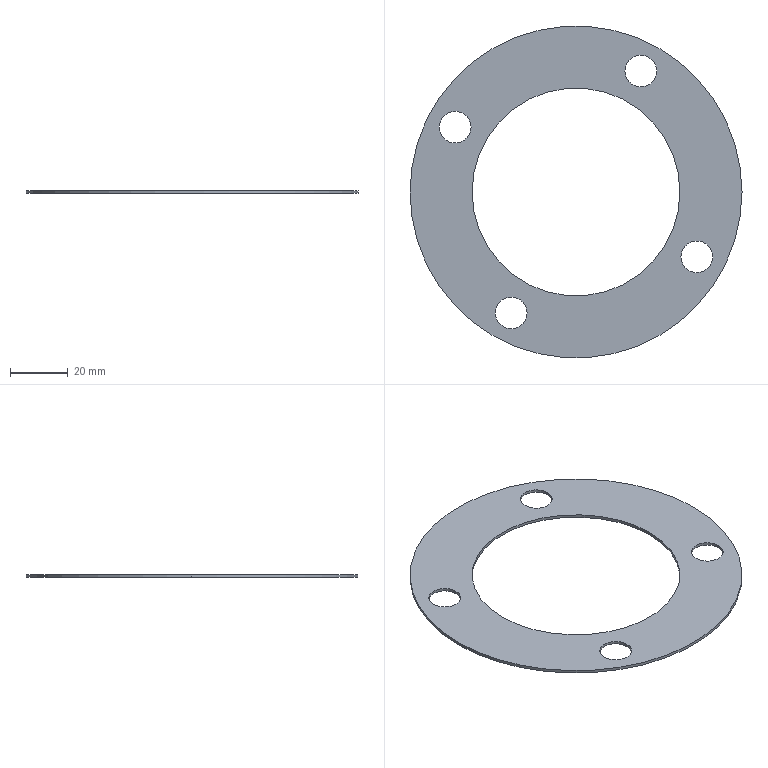Part | SolidWorks | features BaseBody 1 | 1 solid | 14 faces | box 115 x 115 x 1 mm | volume 5935 mm3 | cylinder 12 | plane 2 | commonest cylinder face diameters 11 x8 72 x2 115 x2
STEP:
#1=CARTESIAN_POINT('',(47.934,-43.434,0.));
#2=VERTEX_POINT('',#1);
#3=CARTESIAN_POINT('',(58.934,-43.434,0.));
#4=VERTEX_POINT('',#3);
#5=CARTESIAN_POINT('',(53.434,-43.434,0.));
#6=DIRECTION('',(0.,0.,1.));
#7=DIRECTION('',(1.,0.,0.));
#8=AXIS2_PLACEMENT_3D('',#5,#6,#7);
#9=CIRCLE('',#8,5.5);
#10=EDGE_CURVE('',#2,#4,#9,.T.);
#11=ORIENTED_EDGE('',*,*,#10,.F.);
#12=CARTESIAN_POINT('',(47.934,-43.434,1.));
#13=VERTEX_POINT('',#12);
#14=CARTESIAN_POINT('',(47.934,-43.434,0.));
#15=DIRECTION('',(0.,0.,1.));
#16=VECTOR('',#15,1000.);
#17=LINE('',#14,#16);
#18=EDGE_CURVE('',#2,#13,#17,.T.);
#19=ORIENTED_EDGE('',*,*,#18,.T.);
#20=CARTESIAN_POINT('',(58.934,-43.434,1.));
#21=VERTEX_POINT('',#20);
#22=CARTESIAN_POINT('',(53.434,-43.434,1.));
#23=DIRECTION('',(0.,0.,-1.));
#24=DIRECTION('',(1.,0.,0.));
#25=AXIS2_PLACEMENT_3D('',#22,#23,#24);
#26=CIRCLE('',#25,5.5);
#27=EDGE_CURVE('',#21,#13,#26,.T.);
#28=ORIENTED_EDGE('',*,*,#27,.F.);
#29=CARTESIAN_POINT('',(58.934,-43.434,0.));
#30=DIRECTION('',(0.,0.,1.));
#31=VECTOR('',#30,1000.);
#32=LINE('',#29,#31);
#33=EDGE_CURVE('',#4,#21,#32,.T.);
#34=ORIENTED_EDGE('',*,*,#33,.F.);
#35=EDGE_LOOP('',(#11,#19,#28,#34));
#36=FACE_OUTER_BOUND('',#35,.T.);
#37=CARTESIAN_POINT('',(53.434,-43.434,0.));
#38=DIRECTION('',(0.,0.,1.));
#39=DIRECTION('',(1.,0.,0.));
#40=AXIS2_PLACEMENT_3D('',#37,#38,#39);
#41=CYLINDRICAL_SURFACE('',#40,5.5);
#42=ADVANCED_FACE('',(#36),#41,.F.);
#43=CARTESIAN_POINT('',(112.242,-24.019,0.));
#44=VERTEX_POINT('',#43);
#45=CARTESIAN_POINT('',(123.242,-24.019,0.));
#46=VERTEX_POINT('',#45);
#47=CARTESIAN_POINT('',(117.742,-24.019,0.));
#48=DIRECTION('',(0.,0.,1.));
#49=DIRECTION('',(1.,0.,0.));
#50=AXIS2_PLACEMENT_3D('',#47,#48,#49);
#51=CIRCLE('',#50,5.5);
#52=EDGE_CURVE('',#44,#46,#51,.T.);
#53=ORIENTED_EDGE('',*,*,#52,.F.);
#54=CARTESIAN_POINT('',(112.242,-24.019,1.));
#55=VERTEX_POINT('',#54);
#56=CARTESIAN_POINT('',(112.242,-24.019,0.));
#57=DIRECTION('',(0.,0.,1.));
#58=VECTOR('',#57,1000.);
#59=LINE('',#56,#58);
#60=EDGE_CURVE('',#44,#55,#59,.T.);
#61=ORIENTED_EDGE('',*,*,#60,.T.);
#62=CARTESIAN_POINT('',(123.242,-24.019,1.));
#63=VERTEX_POINT('',#62);
#64=CARTESIAN_POINT('',(117.742,-24.019,1.));
#65=DIRECTION('',(0.,0.,-1.));
#66=DIRECTION('',(1.,0.,0.));
#67=AXIS2_PLACEMENT_3D('',#64,#65,#66);
#68=CIRCLE('',#67,5.5);
#69=EDGE_CURVE('',#63,#55,#68,.T.);
#70=ORIENTED_EDGE('',*,*,#69,.F.);
#71=CARTESIAN_POINT('',(123.242,-24.019,0.));
#72=DIRECTION('',(0.,0.,1.));
#73=VECTOR('',#72,1000.);
#74=LINE('',#71,#73);
#75=EDGE_CURVE('',#46,#63,#74,.T.);
#76=ORIENTED_EDGE('',*,*,#75,.F.);
#77=EDGE_LOOP('',(#53,#61,#70,#76));
#78=FACE_OUTER_BOUND('',#77,.T.);
#79=CARTESIAN_POINT('',(117.742,-24.019,0.));
#80=DIRECTION('',(0.,0.,1.));
#81=DIRECTION('',(1.,0.,0.));
#82=AXIS2_PLACEMENT_3D('',#79,#80,#81);
#83=CYLINDRICAL_SURFACE('',#82,5.5);
#84=ADVANCED_FACE('',(#78),#83,.F.);
#85=CARTESIAN_POINT('',(92.828,40.289,0.));
#86=VERTEX_POINT('',#85);
#87=CARTESIAN_POINT('',(103.828,40.289,0.));
#88=VERTEX_POINT('',#87);
#89=CARTESIAN_POINT('',(98.328,40.289,0.));
#90=DIRECTION('',(0.,0.,1.));
#91=DIRECTION('',(1.,0.,0.));
#92=AXIS2_PLACEMENT_3D('',#89,#90,#91);
#93=CIRCLE('',#92,5.5);
#94=EDGE_CURVE('',#86,#88,#93,.T.);
#95=ORIENTED_EDGE('',*,*,#94,.F.);
#96=CARTESIAN_POINT('',(92.828,40.289,1.));
#97=VERTEX_POINT('',#96);
#98=CARTESIAN_POINT('',(92.828,40.289,0.));
#99=DIRECTION('',(0.,0.,1.));
#100=VECTOR('',#99,1000.);
#101=LINE('',#98,#100);
#102=EDGE_CURVE('',#86,#97,#101,.T.);
#103=ORIENTED_EDGE('',*,*,#102,.T.);
#104=CARTESIAN_POINT('',(103.828,40.289,1.));
#105=VERTEX_POINT('',#104);
#106=CARTESIAN_POINT('',(98.328,40.289,1.));
#107=DIRECTION('',(0.,0.,-1.));
#108=DIRECTION('',(1.,0.,0.));
#109=AXIS2_PLACEMENT_3D('',#106,#107,#108);
#110=CIRCLE('',#109,5.5);
#111=EDGE_CURVE('',#105,#97,#110,.T.);
#112=ORIENTED_EDGE('',*,*,#111,.F.);
#113=CARTESIAN_POINT('',(103.828,40.289,0.));
#114=DIRECTION('',(0.,0.,1.));
#115=VECTOR('',#114,1000.);
#116=LINE('',#113,#115);
#117=EDGE_CURVE('',#88,#105,#116,.T.);
#118=ORIENTED_EDGE('',*,*,#117,.F.);
#119=EDGE_LOOP('',(#95,#103,#112,#118));
#120=FACE_OUTER_BOUND('',#119,.T.);
#121=CARTESIAN_POINT('',(98.328,40.289,0.));
#122=DIRECTION('',(0.,0.,1.));
#123=DIRECTION('',(1.,0.,0.));
#124=AXIS2_PLACEMENT_3D('',#121,#122,#123);
#125=CYLINDRICAL_SURFACE('',#124,5.5);
#126=ADVANCED_FACE('',(#120),#125,.F.);
#127=CARTESIAN_POINT('',(28.519,20.874,0.));
#128=VERTEX_POINT('',#127);
#129=CARTESIAN_POINT('',(39.519,20.874,0.));
#130=VERTEX_POINT('',#129);
#131=CARTESIAN_POINT('',(34.019,20.874,0.));
#132=DIRECTION('',(0.,0.,1.));
#133=DIRECTION('',(1.,0.,0.));
#134=AXIS2_PLACEMENT_3D('',#131,#132,#133);
#135=CIRCLE('',#134,5.5);
#136=EDGE_CURVE('',#128,#130,#135,.T.);
#137=ORIENTED_EDGE('',*,*,#136,.F.);
#138=CARTESIAN_POINT('',(28.519,20.874,1.));
#139=VERTEX_POINT('',#138);
#140=CARTESIAN_POINT('',(28.519,20.874,0.));
#141=DIRECTION('',(0.,0.,1.));
#142=VECTOR('',#141,1000.);
#143=LINE('',#140,#142);
#144=EDGE_CURVE('',#128,#139,#143,.T.);
#145=ORIENTED_EDGE('',*,*,#144,.T.);
#146=CARTESIAN_POINT('',(39.519,20.874,1.));
#147=VERTEX_POINT('',#146);
#148=CARTESIAN_POINT('',(34.019,20.874,1.));
#149=DIRECTION('',(0.,0.,-1.));
#150=DIRECTION('',(1.,0.,0.));
#151=AXIS2_PLACEMENT_3D('',#148,#149,#150);
#152=CIRCLE('',#151,5.5);
#153=EDGE_CURVE('',#147,#139,#152,.T.);
#154=ORIENTED_EDGE('',*,*,#153,.F.);
#155=CARTESIAN_POINT('',(39.519,20.874,0.));
#156=DIRECTION('',(0.,0.,1.));
#157=VECTOR('',#156,1000.);
#158=LINE('',#155,#157);
#159=EDGE_CURVE('',#130,#147,#158,.T.);
#160=ORIENTED_EDGE('',*,*,#159,.F.);
#161=EDGE_LOOP('',(#137,#145,#154,#160));
#162=FACE_OUTER_BOUND('',#161,.T.);
#163=CARTESIAN_POINT('',(34.019,20.874,0.));
#164=DIRECTION('',(0.,0.,1.));
#165=DIRECTION('',(1.,0.,0.));
#166=AXIS2_PLACEMENT_3D('',#163,#164,#165);
#167=CYLINDRICAL_SURFACE('',#166,5.5);
#168=ADVANCED_FACE('',(#162),#167,.F.);
#169=CARTESIAN_POINT('',(39.881,-1.573,0.));
#170=VERTEX_POINT('',#169);
#171=CARTESIAN_POINT('',(111.881,-1.573,0.));
#172=VERTEX_POINT('',#171);
#173=CARTESIAN_POINT('',(75.881,-1.573,0.));
#174=DIRECTION('',(0.,0.,1.));
#175=DIRECTION('',(1.,0.,0.));
#176=AXIS2_PLACEMENT_3D('',#173,#174,#175);
#177=CIRCLE('',#176,36.);
#178=EDGE_CURVE('',#170,#172,#177,.T.);
#179=ORIENTED_EDGE('',*,*,#178,.F.);
#180=CARTESIAN_POINT('',(39.881,-1.573,1.));
#181=VERTEX_POINT('',#180);
#182=CARTESIAN_POINT('',(39.881,-1.573,0.));
#183=DIRECTION('',(0.,0.,1.));
#184=VECTOR('',#183,1000.);
#185=LINE('',#182,#184);
#186=EDGE_CURVE('',#170,#181,#185,.T.);
#187=ORIENTED_EDGE('',*,*,#186,.T.);
#188=CARTESIAN_POINT('',(111.881,-1.573,1.));
#189=VERTEX_POINT('',#188);
#190=CARTESIAN_POINT('',(75.881,-1.573,1.));
#191=DIRECTION('',(0.,0.,-1.));
#192=DIRECTION('',(1.,0.,0.));
#193=AXIS2_PLACEMENT_3D('',#190,#191,#192);
#194=CIRCLE('',#193,36.);
#195=EDGE_CURVE('',#189,#181,#194,.T.);
#196=ORIENTED_EDGE('',*,*,#195,.F.);
#197=CARTESIAN_POINT('',(111.881,-1.573,0.));
#198=DIRECTION('',(0.,0.,1.));
#199=VECTOR('',#198,1000.);
#200=LINE('',#197,#199);
#201=EDGE_CURVE('',#172,#189,#200,.T.);
#202=ORIENTED_EDGE('',*,*,#201,.F.);
#203=EDGE_LOOP('',(#179,#187,#196,#202));
#204=FACE_OUTER_BOUND('',#203,.T.);
#205=CARTESIAN_POINT('',(75.881,-1.573,0.));
#206=DIRECTION('',(0.,0.,1.));
#207=DIRECTION('',(1.,0.,0.));
#208=AXIS2_PLACEMENT_3D('',#205,#206,#207);
#209=CYLINDRICAL_SURFACE('',#208,36.);
#210=ADVANCED_FACE('',(#204),#209,.F.);
#211=CARTESIAN_POINT('',(133.381,-1.573,0.));
#212=VERTEX_POINT('',#211);
#213=CARTESIAN_POINT('',(18.381,-1.573,0.));
#214=VERTEX_POINT('',#213);
#215=CARTESIAN_POINT('',(75.881,-1.573,0.));
#216=DIRECTION('',(0.,0.,1.));
#217=DIRECTION('',(1.,0.,0.));
#218=AXIS2_PLACEMENT_3D('',#215,#216,#217);
#219=CIRCLE('',#218,57.5);
#220=EDGE_CURVE('',#212,#214,#219,.T.);
#221=ORIENTED_EDGE('',*,*,#220,.T.);
#222=CARTESIAN_POINT('',(18.381,-1.573,1.));
#223=VERTEX_POINT('',#222);
#224=CARTESIAN_POINT('',(18.381,-1.573,0.));
#225=DIRECTION('',(0.,0.,1.));
#226=VECTOR('',#225,1000.);
#227=LINE('',#224,#226);
#228=EDGE_CURVE('',#214,#223,#227,.T.);
#229=ORIENTED_EDGE('',*,*,#228,.T.);
#230=CARTESIAN_POINT('',(133.381,-1.573,1.));
#231=VERTEX_POINT('',#230);
#232=CARTESIAN_POINT('',(75.881,-1.573,1.));
#233=DIRECTION('',(0.,0.,1.));
#234=DIRECTION('',(1.,0.,0.));
#235=AXIS2_PLACEMENT_3D('',#232,#233,#234);
#236=CIRCLE('',#235,57.5);
#237=EDGE_CURVE('',#231,#223,#236,.T.);
#238=ORIENTED_EDGE('',*,*,#237,.F.);
#239=CARTESIAN_POINT('',(133.381,-1.573,0.));
#240=DIRECTION('',(0.,0.,1.));
#241=VECTOR('',#240,1000.);
#242=LINE('',#239,#241);
#243=EDGE_CURVE('',#212,#231,#242,.T.);
#244=ORIENTED_EDGE('',*,*,#243,.F.);
#245=EDGE_LOOP('',(#221,#229,#238,#244));
#246=FACE_OUTER_BOUND('',#245,.T.);
#247=CARTESIAN_POINT('',(75.881,-1.573,0.));
#248=DIRECTION('',(0.,0.,1.));
#249=DIRECTION('',(1.,0.,0.));
#250=AXIS2_PLACEMENT_3D('',#247,#248,#249);
#251=CYLINDRICAL_SURFACE('',#250,57.5);
#252=ADVANCED_FACE('',(#246),#251,.T.);
#253=ORIENTED_EDGE('',*,*,#27,.T.);
#254=CARTESIAN_POINT('',(53.434,-43.434,1.));
#255=DIRECTION('',(0.,0.,-1.));
#256=DIRECTION('',(1.,0.,0.));
#257=AXIS2_PLACEMENT_3D('',#254,#255,#256);
#258=CIRCLE('',#257,5.5);
#259=EDGE_CURVE('',#13,#21,#258,.T.);
#260=ORIENTED_EDGE('',*,*,#259,.T.);
#261=EDGE_LOOP('',(#253,#260));
#262=FACE_BOUND('',#261,.T.);
#263=ORIENTED_EDGE('',*,*,#69,.T.);
#264=CARTESIAN_POINT('',(117.742,-24.019,1.));
#265=DIRECTION('',(0.,0.,-1.));
#266=DIRECTION('',(1.,0.,0.));
#267=AXIS2_PLACEMENT_3D('',#264,#265,#266);
#268=CIRCLE('',#267,5.5);
#269=EDGE_CURVE('',#55,#63,#268,.T.);
#270=ORIENTED_EDGE('',*,*,#269,.T.);
#271=EDGE_LOOP('',(#263,#270));
#272=FACE_BOUND('',#271,.T.);
#273=ORIENTED_EDGE('',*,*,#111,.T.);
#274=CARTESIAN_POINT('',(98.328,40.289,1.));
#275=DIRECTION('',(0.,0.,-1.));
#276=DIRECTION('',(1.,0.,0.));
#277=AXIS2_PLACEMENT_3D('',#274,#275,#276);
#278=CIRCLE('',#277,5.5);
#279=EDGE_CURVE('',#97,#105,#278,.T.);
#280=ORIENTED_EDGE('',*,*,#279,.T.);
#281=EDGE_LOOP('',(#273,#280));
#282=FACE_BOUND('',#281,.T.);
#283=ORIENTED_EDGE('',*,*,#153,.T.);
#284=CARTESIAN_POINT('',(34.019,20.874,1.));
#285=DIRECTION('',(0.,0.,-1.));
#286=DIRECTION('',(1.,0.,0.));
#287=AXIS2_PLACEMENT_3D('',#284,#285,#286);
#288=CIRCLE('',#287,5.5);
#289=EDGE_CURVE('',#139,#147,#288,.T.);
#290=ORIENTED_EDGE('',*,*,#289,.T.);
#291=EDGE_LOOP('',(#283,#290));
#292=FACE_BOUND('',#291,.T.);
#293=ORIENTED_EDGE('',*,*,#195,.T.);
#294=CARTESIAN_POINT('',(75.881,-1.573,1.));
#295=DIRECTION('',(0.,0.,-1.));
#296=DIRECTION('',(1.,0.,0.));
#297=AXIS2_PLACEMENT_3D('',#294,#295,#296);
#298=CIRCLE('',#297,36.);
#299=EDGE_CURVE('',#181,#189,#298,.T.);
#300=ORIENTED_EDGE('',*,*,#299,.T.);
#301=EDGE_LOOP('',(#293,#300));
#302=FACE_BOUND('',#301,.T.);
#303=ORIENTED_EDGE('',*,*,#237,.T.);
#304=CARTESIAN_POINT('',(75.881,-1.573,1.));
#305=DIRECTION('',(0.,0.,1.));
#306=DIRECTION('',(1.,0.,0.));
#307=AXIS2_PLACEMENT_3D('',#304,#305,#306);
#308=CIRCLE('',#307,57.5);
#309=EDGE_CURVE('',#223,#231,#308,.T.);
#310=ORIENTED_EDGE('',*,*,#309,.T.);
#311=EDGE_LOOP('',(#303,#310));
#312=FACE_OUTER_BOUND('',#311,.T.);
#313=CARTESIAN_POINT('',(75.881,-1.573,1.));
#314=DIRECTION('',(0.,0.,1.));
#315=DIRECTION('',(1.,0.,0.));
#316=AXIS2_PLACEMENT_3D('',#313,#314,#315);
#317=PLANE('',#316);
#318=ADVANCED_FACE('',(#262,#272,#282,#292,#302,#312),#317,.T.);
#319=ORIENTED_EDGE('',*,*,#18,.F.);
#320=CARTESIAN_POINT('',(53.434,-43.434,0.));
#321=DIRECTION('',(0.,0.,1.));
#322=DIRECTION('',(1.,0.,0.));
#323=AXIS2_PLACEMENT_3D('',#320,#321,#322);
#324=CIRCLE('',#323,5.5);
#325=EDGE_CURVE('',#4,#2,#324,.T.);
#326=ORIENTED_EDGE('',*,*,#325,.F.);
#327=ORIENTED_EDGE('',*,*,#33,.T.);
#328=ORIENTED_EDGE('',*,*,#259,.F.);
#329=EDGE_LOOP('',(#319,#326,#327,#328));
#330=FACE_OUTER_BOUND('',#329,.T.);
#331=CARTESIAN_POINT('',(53.434,-43.434,0.));
#332=DIRECTION('',(0.,0.,1.));
#333=DIRECTION('',(1.,0.,0.));
#334=AXIS2_PLACEMENT_3D('',#331,#332,#333);
#335=CYLINDRICAL_SURFACE('',#334,5.5);
#336=ADVANCED_FACE('',(#330),#335,.F.);
#337=ORIENTED_EDGE('',*,*,#60,.F.);
#338=CARTESIAN_POINT('',(117.742,-24.019,0.));
#339=DIRECTION('',(0.,0.,1.));
#340=DIRECTION('',(1.,0.,0.));
#341=AXIS2_PLACEMENT_3D('',#338,#339,#340);
#342=CIRCLE('',#341,5.5);
#343=EDGE_CURVE('',#46,#44,#342,.T.);
#344=ORIENTED_EDGE('',*,*,#343,.F.);
#345=ORIENTED_EDGE('',*,*,#75,.T.);
#346=ORIENTED_EDGE('',*,*,#269,.F.);
#347=EDGE_LOOP('',(#337,#344,#345,#346));
#348=FACE_OUTER_BOUND('',#347,.T.);
#349=CARTESIAN_POINT('',(117.742,-24.019,0.));
#350=DIRECTION('',(0.,0.,1.));
#351=DIRECTION('',(1.,0.,0.));
#352=AXIS2_PLACEMENT_3D('',#349,#350,#351);
#353=CYLINDRICAL_SURFACE('',#352,5.5);
#354=ADVANCED_FACE('',(#348),#353,.F.);
#355=ORIENTED_EDGE('',*,*,#102,.F.);
#356=CARTESIAN_POINT('',(98.328,40.289,0.));
#357=DIRECTION('',(0.,0.,1.));
#358=DIRECTION('',(1.,0.,0.));
#359=AXIS2_PLACEMENT_3D('',#356,#357,#358);
#360=CIRCLE('',#359,5.5);
#361=EDGE_CURVE('',#88,#86,#360,.T.);
#362=ORIENTED_EDGE('',*,*,#361,.F.);
#363=ORIENTED_EDGE('',*,*,#117,.T.);
#364=ORIENTED_EDGE('',*,*,#279,.F.);
#365=EDGE_LOOP('',(#355,#362,#363,#364));
#366=FACE_OUTER_BOUND('',#365,.T.);
#367=CARTESIAN_POINT('',(98.328,40.289,0.));
#368=DIRECTION('',(0.,0.,1.));
#369=DIRECTION('',(1.,0.,0.));
#370=AXIS2_PLACEMENT_3D('',#367,#368,#369);
#371=CYLINDRICAL_SURFACE('',#370,5.5);
#372=ADVANCED_FACE('',(#366),#371,.F.);
#373=ORIENTED_EDGE('',*,*,#144,.F.);
#374=CARTESIAN_POINT('',(34.019,20.874,0.));
#375=DIRECTION('',(0.,0.,1.));
#376=DIRECTION('',(1.,0.,0.));
#377=AXIS2_PLACEMENT_3D('',#374,#375,#376);
#378=CIRCLE('',#377,5.5);
#379=EDGE_CURVE('',#130,#128,#378,.T.);
#380=ORIENTED_EDGE('',*,*,#379,.F.);
#381=ORIENTED_EDGE('',*,*,#159,.T.);
#382=ORIENTED_EDGE('',*,*,#289,.F.);
#383=EDGE_LOOP('',(#373,#380,#381,#382));
#384=FACE_OUTER_BOUND('',#383,.T.);
#385=CARTESIAN_POINT('',(34.019,20.874,0.));
#386=DIRECTION('',(0.,0.,1.));
#387=DIRECTION('',(1.,0.,0.));
#388=AXIS2_PLACEMENT_3D('',#385,#386,#387);
#389=CYLINDRICAL_SURFACE('',#388,5.5);
#390=ADVANCED_FACE('',(#384),#389,.F.);
#391=ORIENTED_EDGE('',*,*,#186,.F.);
#392=CARTESIAN_POINT('',(75.881,-1.573,0.));
#393=DIRECTION('',(0.,0.,1.));
#394=DIRECTION('',(1.,0.,0.));
#395=AXIS2_PLACEMENT_3D('',#392,#393,#394);
#396=CIRCLE('',#395,36.);
#397=EDGE_CURVE('',#172,#170,#396,.T.);
#398=ORIENTED_EDGE('',*,*,#397,.F.);
#399=ORIENTED_EDGE('',*,*,#201,.T.);
#400=ORIENTED_EDGE('',*,*,#299,.F.);
#401=EDGE_LOOP('',(#391,#398,#399,#400));
#402=FACE_OUTER_BOUND('',#401,.T.);
#403=CARTESIAN_POINT('',(75.881,-1.573,0.));
#404=DIRECTION('',(0.,0.,1.));
#405=DIRECTION('',(1.,0.,0.));
#406=AXIS2_PLACEMENT_3D('',#403,#404,#405);
#407=CYLINDRICAL_SURFACE('',#406,36.);
#408=ADVANCED_FACE('',(#402),#407,.F.);
#409=ORIENTED_EDGE('',*,*,#228,.F.);
#410=CARTESIAN_POINT('',(75.881,-1.573,0.));
#411=DIRECTION('',(0.,0.,1.));
#412=DIRECTION('',(1.,0.,0.));
#413=AXIS2_PLACEMENT_3D('',#410,#411,#412);
#414=CIRCLE('',#413,57.5);
#415=EDGE_CURVE('',#214,#212,#414,.T.);
#416=ORIENTED_EDGE('',*,*,#415,.T.);
#417=ORIENTED_EDGE('',*,*,#243,.T.);
#418=ORIENTED_EDGE('',*,*,#309,.F.);
#419=EDGE_LOOP('',(#409,#416,#417,#418));
#420=FACE_OUTER_BOUND('',#419,.T.);
#421=CARTESIAN_POINT('',(75.881,-1.573,0.));
#422=DIRECTION('',(0.,0.,1.));
#423=DIRECTION('',(1.,0.,0.));
#424=AXIS2_PLACEMENT_3D('',#421,#422,#423);
#425=CYLINDRICAL_SURFACE('',#424,57.5);
#426=ADVANCED_FACE('',(#420),#425,.T.);
#427=ORIENTED_EDGE('',*,*,#325,.T.);
#428=ORIENTED_EDGE('',*,*,#10,.T.);
#429=EDGE_LOOP('',(#427,#428));
#430=FACE_BOUND('',#429,.T.);
#431=ORIENTED_EDGE('',*,*,#343,.T.);
#432=ORIENTED_EDGE('',*,*,#52,.T.);
#433=EDGE_LOOP('',(#431,#432));
#434=FACE_BOUND('',#433,.T.);
#435=ORIENTED_EDGE('',*,*,#361,.T.);
#436=ORIENTED_EDGE('',*,*,#94,.T.);
#437=EDGE_LOOP('',(#435,#436));
#438=FACE_BOUND('',#437,.T.);
#439=ORIENTED_EDGE('',*,*,#379,.T.);
#440=ORIENTED_EDGE('',*,*,#136,.T.);
#441=EDGE_LOOP('',(#439,#440));
#442=FACE_BOUND('',#441,.T.);
#443=ORIENTED_EDGE('',*,*,#397,.T.);
#444=ORIENTED_EDGE('',*,*,#178,.T.);
#445=EDGE_LOOP('',(#443,#444));
#446=FACE_BOUND('',#445,.T.);
#447=ORIENTED_EDGE('',*,*,#220,.F.);
#448=ORIENTED_EDGE('',*,*,#415,.F.);
#449=EDGE_LOOP('',(#447,#448));
#450=FACE_OUTER_BOUND('',#449,.T.);
#451=CARTESIAN_POINT('',(75.881,-1.573,0.));
#452=DIRECTION('',(0.,0.,1.));
#453=DIRECTION('',(1.,0.,0.));
#454=AXIS2_PLACEMENT_3D('',#451,#452,#453);
#455=PLANE('',#454);
#456=ADVANCED_FACE('',(#430,#434,#438,#442,#446,#450),#455,.F.);
#457=CLOSED_SHELL('',(#42,#84,#126,#168,#210,#252,#318,#336,#354,#372,#390,#408,#426,#456));
#458=MANIFOLD_SOLID_BREP('',#457);
#459=CARTESIAN_POINT('',(0.,0.,0.));
#460=DIRECTION('',(0.,0.,1.));
#461=DIRECTION('',(1.,0.,0.));
#462=AXIS2_PLACEMENT_3D('',#459,#460,#461);
#463=(LENGTH_UNIT()NAMED_UNIT(*)SI_UNIT(.MILLI.,.METRE.));
#464=UNCERTAINTY_MEASURE_WITH_UNIT(LENGTH_MEASURE(0.00001),#463,'','');
#465=(NAMED_UNIT(*)PLANE_ANGLE_UNIT()SI_UNIT($,.RADIAN.));
#466=(NAMED_UNIT(*)SI_UNIT($,.STERADIAN.)SOLID_ANGLE_UNIT());
#467=(GEOMETRIC_REPRESENTATION_CONTEXT(3)GLOBAL_UNCERTAINTY_ASSIGNED_CONTEXT((#464))GLOBAL_UNIT_ASSIGNED_CONTEXT((#463,#465,#466))REPRESENTATION_CONTEXT('',''));
#468=ADVANCED_BREP_SHAPE_REPRESENTATION('',(#458,#462),#467);